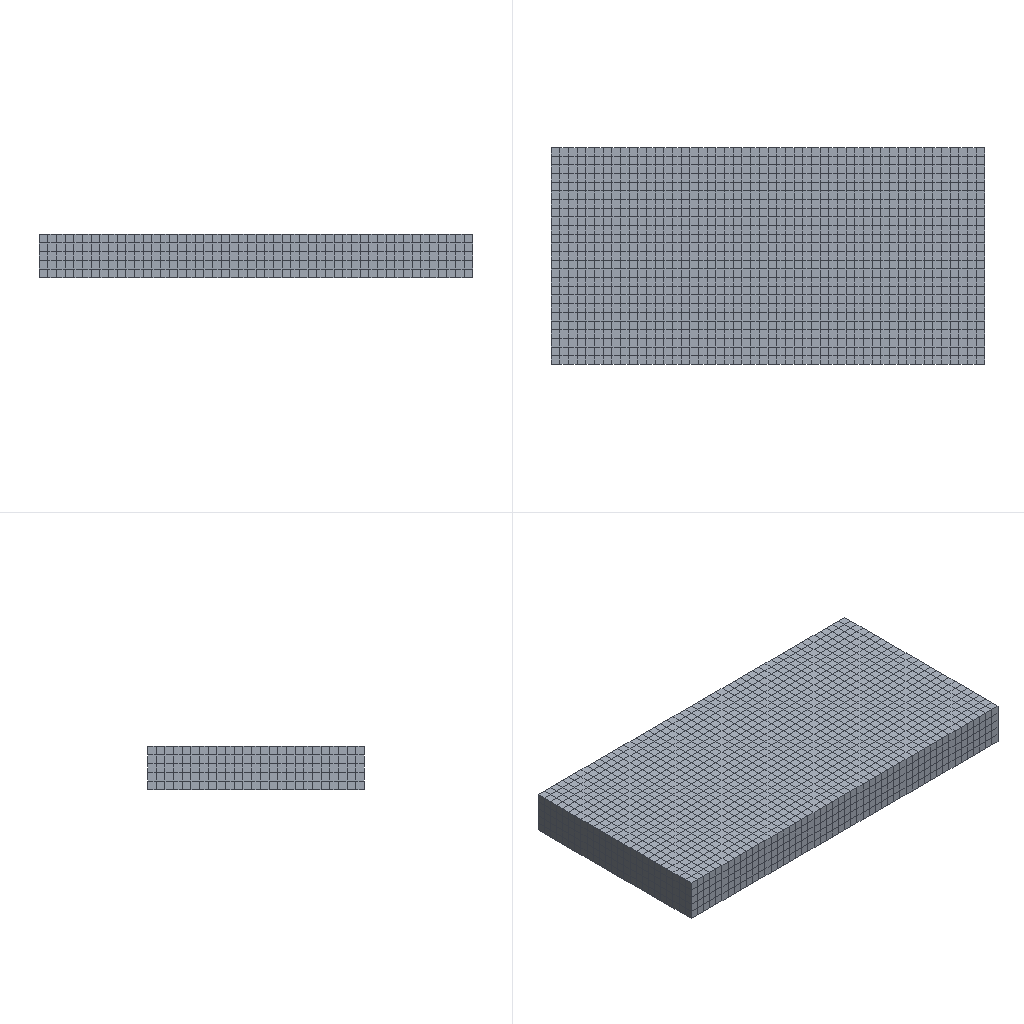Simulation study | abaqus
Abaqus input file, long lists of numbers shortened:
*Heading
** Job name: deck-3 Model name: Model-1-Copy2
** Generated by: Abaqus/CAE 2024
*Preprint, echo=NO, model=NO, history=NO, contact=NO
**
** PARTS
**
*Part, name=Part-1
*Node
      1,           0.,         -25.,           5.
      2,           0.,         -24.,           5.
** (7954 more lines like these left out)
*Element, type=C3D8R
   1,  157,  158,  184,  183,    1,    2,   28,   27
   2,  158,  159,  185,  184,    2,    3,   29,   28
** (6248 more lines like these left out)
*Nset, nset=Set-1, generate
    1,  7956,     1
*Elset, elset=Set-1, generate
    1,  6250,     1
** Section: Section-1
*Solid Section, elset=Set-1, material=Material-1
,
*End Part
**
*Part, name=tool
*Node
      1,           5.,         10.5,           2.
      2,           5.,   3.762,           2.
** (472 more lines like these left out)
*Element, type=R3D4
 1,   1,   9, 109,  40
 2,   9,  10, 110, 109
** (470 more lines like these left out)
*Node
    475,           5.,         10.5,           1.
*Nset, nset=tool-RefPt_, internal
475,
*Elset, elset=tool, generate
   1,  472,    1
*End Part
**
**
** ASSEMBLY
**
*Assembly, name=Assembly
**
*Instance, name=Part-1-1, part=Part-1
*End Instance
**
*Instance, name=tool-1, part=tool
         50.,        -11.5,           1.
         50.,        -11.5,           1., 51.,        -11.5,           1., 90.
*End Instance
**
*Instance, name=tool-1-lin-2-1, part=tool
         50.,         -5.5,           1.
         50.,         -5.5,           1., 51.,         -5.5,           1., 90.
*End Instance
**
*Instance, name=tool-1-lin-2-1-1, part=tool
         50.,        -17.5,           1.
         50.,        -17.5,           1., 51.,        -17.5,           1., 90.
*End Instance
**
*Nset, nset=Set-1, instance=Part-1-1
  131,  132,  133,  134,  135,  136,  137,  138,  139,  140,  141,  142,  143,  144,  145,  146
  147,  148,  149,  150,  151,  152,  153,  154,  155,  156,  287,  288,  289,  290,  291,  292
** (81 more lines like these left out)
*Elset, elset=Set-1, instance=Part-1-1
  101,  102,  103,  104,  105,  106,  107,  108,  109,  110,  111,  112,  113,  114,  115,  116
  117,  118,  119,  120,  121,  122,  123,  124,  125,  226,  227,  228,  229,  230,  231,  232
** (77 more lines like these left out)
*Nset, nset=Set-3, instance=tool-1-lin-2-1-1
 475,
*Nset, nset=Set-4, instance=tool-1
 475,
*Nset, nset=Set-5, instance=tool-1-lin-2-1
 475,
*Nset, nset=s_Set-2, instance=Part-1-1, generate
    1,  7956,     1
*Elset, elset=s_Set-2, instance=Part-1-1, generate
    1,  6250,     1
*Elset, elset=_m_Surf-1_SPOS, internal, instance=tool-1-lin-2-1-1, generate
   1,  472,    1
*Surface, type=ELEMENT, name=m_Surf-1
_m_Surf-1_SPOS, SPOS
*Elset, elset=_m_Surf-2_SPOS, internal, instance=tool-1, generate
   1,  472,    1
*Surface, type=ELEMENT, name=m_Surf-2
_m_Surf-2_SPOS, SPOS
*Elset, elset=_m_Surf-3_SPOS, internal, instance=tool-1-lin-2-1, generate
   1,  472,    1
*Surface, type=ELEMENT, name=m_Surf-3
_m_Surf-3_SPOS, SPOS
*Surface, type=NODE, name=s_Set-2_CNS_, internal
s_Set-2, 1.
*Rigid Body, ref node=tool-1.tool-RefPt_, elset=tool-1.tool
*Rigid Body, ref node=tool-1-lin-2-1.tool-RefPt_, elset=tool-1-lin-2-1.tool
*Rigid Body, ref node=tool-1-lin-2-1-1.tool-RefPt_, elset=tool-1-lin-2-1-1.tool
*End Assembly
**
** MATERIALS
**
*Material, name=Material-1
*Damage Initiation, criterion=SHEAR
 0.1,0.,0.
*Damage Evolution, type=DISPLACEMENT
 1e-05,
*Density
 2.8e-09,
*Elastic
72000., 0.3
*Plastic
200.,0.
**
** INTERACTION PROPERTIES
**
*Surface Interaction, name=IntProp-1
*Friction
 0.2,
*Surface Behavior, pressure-overclosure=HARD
** ----------------------------------------------------------------
**
** STEP: Step-1
**
*Step, name=Step-1, nlgeom=YES
*Dynamic, Explicit
, 0.01
*Bulk Viscosity
0.06, 1.2
** Mass Scaling: Semi-Automatic
**               Whole Model
*Fixed Mass Scaling, factor=500.
**
** BOUNDARY CONDITIONS
**
** Name: BC-fix Type: Symmetry/Antisymmetry/Encastre
*Boundary
Set-1, ENCASTRE
** Name: BC-v1 Type: Velocity/Angular velocity
*Boundary, type=VELOCITY
Set-3, 1, 1, -5600.
Set-3, 2, 2
Set-3, 3, 3
Set-3, 4, 4
Set-3, 5, 5
Set-3, 6, 6
** Name: BC-v2 Type: Velocity/Angular velocity
*Boundary, type=VELOCITY
Set-4, 1, 1
Set-4, 2, 2
Set-4, 3, 3
Set-4, 4, 4
Set-4, 5, 5
Set-4, 6, 6
** Name: BC-v3 Type: Velocity/Angular velocity
*Boundary, type=VELOCITY
Set-5, 1, 1
Set-5, 2, 2
Set-5, 3, 3
Set-5, 4, 4
Set-5, 5, 5
Set-5, 6, 6
**
** INTERACTIONS
**
** Interaction: Int-1
*Contact Pair, interaction=IntProp-1, mechanical constraint=KINEMATIC, cpset=Int-1
m_Surf-1, s_Set-2_CNS_
** Interaction: Int-1-Copy
*Contact Pair, interaction=IntProp-1, mechanical constraint=KINEMATIC, cpset=Int-1-Copy
m_Surf-2, s_Set-2_CNS_
** Interaction: Int-1-Copy2
*Contact Pair, interaction=IntProp-1, mechanical constraint=KINEMATIC, cpset=Int-1-Copy2
m_Surf-3, s_Set-2_CNS_
**
** OUTPUT REQUESTS
**
*Restart, write, number interval=1, time marks=NO
**
** FIELD OUTPUT: F-Output-1
**
*Output, field, number interval=40
*Node Output
A, CF, RF, RM, RT, U, V
*Element Output, directions=YES
E, EVF, LE, MISES, MISESMAX, PE, PEEQ, PEEQVAVG, PEVAVG, S, STATUS, SVAVG
*Contact Output
CDISP, CSTRESS
**
** HISTORY OUTPUT: H-Output-1
**
*Output, history, time interval=2e-07
*Node Output, nset=Set-1
RF1, RF2, RF3
*End Step
** ----------------------------------------------------------------
**
** STEP: Step-2
**
*Step, name=Step-2, nlgeom=YES
*Dynamic, Explicit
, 0.01
*Bulk Viscosity
0.06, 1.2
** Mass Scaling: Semi-Automatic
**               Whole Model
*Fixed Mass Scaling, factor=500.
**
** BOUNDARY CONDITIONS
**
** Name: BC-v1 Type: Velocity/Angular velocity
*Boundary, type=VELOCITY
Set-3, 1, 1
** Name: BC-v2 Type: Velocity/Angular velocity
*Boundary, type=VELOCITY
Set-4, 1, 1, -5600.
**
** OUTPUT REQUESTS
**
*Restart, write, number interval=1, time marks=NO
**
** FIELD OUTPUT: F-Output-1
**
*Output, field, number interval=40
*Node Output
A, CF, RF, RM, RT, U, V
*Element Output, directions=YES
E, EVF, LE, MISES, MISESMAX, PE, PEEQ, PEEQVAVG, PEVAVG, S, STATUS, SVAVG
*Contact Output
CDISP, CSTRESS
**
** HISTORY OUTPUT: H-Output-2
**
*Output, history, time interval=2e-07
*Node Output, nset=Set-3
RF1, RF2, RF3
*End Step
** ----------------------------------------------------------------
**
** STEP: Step-3
**
*Step, name=Step-3, nlgeom=YES
*Dynamic, Explicit
, 0.01
*Bulk Viscosity
0.06, 1.2
** Mass Scaling: Semi-Automatic
**               Whole Model
*Fixed Mass Scaling, factor=500.
**
** BOUNDARY CONDITIONS
**
** Name: BC-v2 Type: Velocity/Angular velocity
*Boundary, type=VELOCITY
Set-4, 1, 1
** Name: BC-v3 Type: Velocity/Angular velocity
*Boundary, type=VELOCITY
Set-5, 1, 1, -5600.
**
** OUTPUT REQUESTS
**
*Restart, write, number interval=1, time marks=NO
**
** FIELD OUTPUT: F-Output-1
**
*Output, field, number interval=40
*Node Output
A, CF, RF, RM, RT, U, V
*Element Output, directions=YES
E, EVF, LE, MISES, MISESMAX, PE, PEEQ, PEEQVAVG, PEVAVG, S, STATUS, SVAVG
*Contact Output
CDISP, CSTRESS
**
** HISTORY OUTPUT: H-Output-3
**
*Output, history, time interval=2e-07
*Node Output, nset=Set-5
RF1, RF2, RF3
*End Step